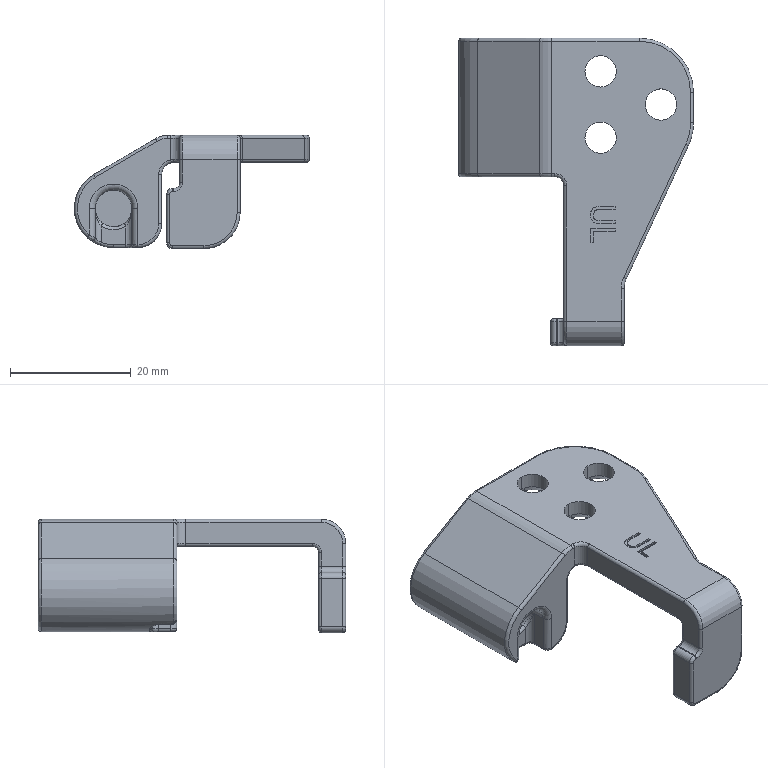Part | NX | features solid 2 | 1 solid | 138 faces | box 38.991 x 50.97 x 18.8 mm | volume 8011 mm3 | cylinder 55 | plane 34 | torus 28 | spline 15 | cone 6 | commonest cylinder face diameters 1 x29 2 x8 5.2 x6 8 x4 6.1 x2 18 x2